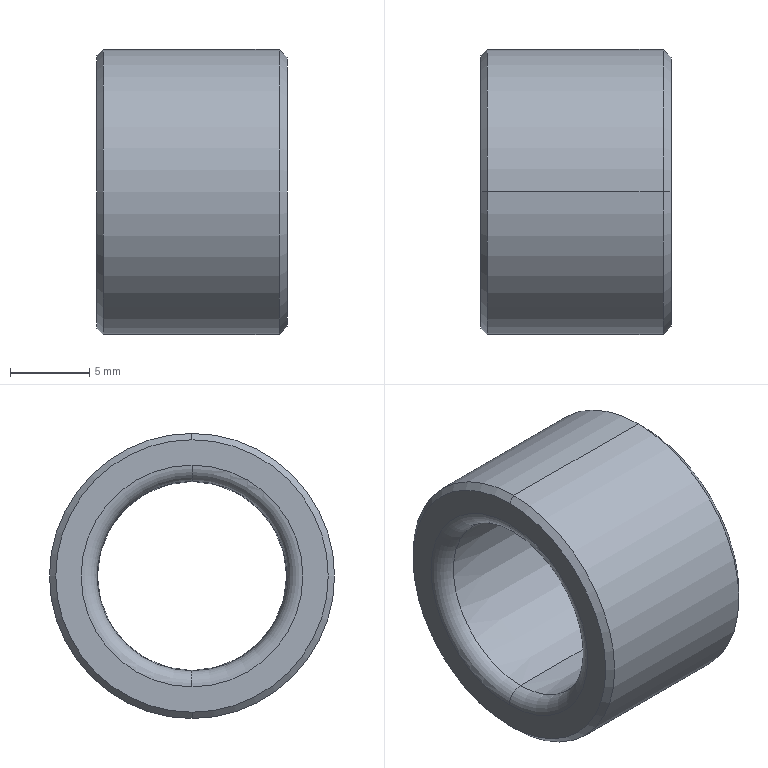Part | STEP file | SHBZ12_12_SHBZ12-100 | 1 solid | 16 faces | box 12 x 18 x 18 mm | volume 1675 mm3 | torus 6 | cone 6 | cylinder 2 | plane 2 | commonest cylinder face diameters 18 x2
STEP:
#1=CARTESIAN_POINT('',(11.,0.,-5.969));
#2=VERTEX_POINT('',#1);
#3=CARTESIAN_POINT('',(12.,0.,-6.969));
#4=VERTEX_POINT('',#3);
#5=CARTESIAN_POINT('',(11.,0.,-6.969));
#6=DIRECTION('',(0.,1.,0.));
#7=DIRECTION('',(0.,0.,1.));
#8=AXIS2_PLACEMENT_3D('',#5,#6,#7);
#9=CIRCLE('',#8,1.);
#10=EDGE_CURVE('',#2,#4,#9,.T.);
#11=ORIENTED_EDGE('',*,*,#10,.F.);
#12=CARTESIAN_POINT('',(11.,0.,5.969));
#13=VERTEX_POINT('',#12);
#14=CARTESIAN_POINT('',(11.,0.,0.));
#15=DIRECTION('',(-1.,0.,0.));
#16=DIRECTION('',(0.,0.,1.));
#17=AXIS2_PLACEMENT_3D('',#14,#15,#16);
#18=CIRCLE('',#17,5.969);
#19=EDGE_CURVE('',#2,#13,#18,.T.);
#20=ORIENTED_EDGE('',*,*,#19,.T.);
#21=CARTESIAN_POINT('',(12.,0.,6.969));
#22=VERTEX_POINT('',#21);
#23=CARTESIAN_POINT('',(11.,0.,6.969));
#24=DIRECTION('',(0.,-1.,0.));
#25=DIRECTION('',(0.,0.,-1.));
#26=AXIS2_PLACEMENT_3D('',#23,#24,#25);
#27=CIRCLE('',#26,1.);
#28=EDGE_CURVE('',#13,#22,#27,.T.);
#29=ORIENTED_EDGE('',*,*,#28,.T.);
#30=CARTESIAN_POINT('',(12.,0.,0.));
#31=DIRECTION('',(-1.,0.,0.));
#32=DIRECTION('',(0.,0.,1.));
#33=AXIS2_PLACEMENT_3D('',#30,#31,#32);
#34=CIRCLE('',#33,6.969);
#35=EDGE_CURVE('',#4,#22,#34,.T.);
#36=ORIENTED_EDGE('',*,*,#35,.F.);
#37=EDGE_LOOP('',(#11,#20,#29,#36));
#38=FACE_OUTER_BOUND('',#37,.T.);
#39=CARTESIAN_POINT('',(11.,0.,0.));
#40=DIRECTION('',(-1.,0.,0.));
#41=DIRECTION('',(0.,0.,1.));
#42=AXIS2_PLACEMENT_3D('',#39,#40,#41);
#43=TOROIDAL_SURFACE('',#42,6.969,1.);
#44=ADVANCED_FACE('',(#38),#43,.T.);
#45=ORIENTED_EDGE('',*,*,#28,.F.);
#46=CARTESIAN_POINT('',(11.,0.,0.));
#47=DIRECTION('',(-1.,0.,0.));
#48=DIRECTION('',(0.,0.,1.));
#49=AXIS2_PLACEMENT_3D('',#46,#47,#48);
#50=CIRCLE('',#49,5.969);
#51=EDGE_CURVE('',#13,#2,#50,.T.);
#52=ORIENTED_EDGE('',*,*,#51,.T.);
#53=ORIENTED_EDGE('',*,*,#10,.T.);
#54=CARTESIAN_POINT('',(12.,0.,0.));
#55=DIRECTION('',(-1.,0.,0.));
#56=DIRECTION('',(0.,0.,1.));
#57=AXIS2_PLACEMENT_3D('',#54,#55,#56);
#58=CIRCLE('',#57,6.969);
#59=EDGE_CURVE('',#22,#4,#58,.T.);
#60=ORIENTED_EDGE('',*,*,#59,.F.);
#61=EDGE_LOOP('',(#45,#52,#53,#60));
#62=FACE_OUTER_BOUND('',#61,.T.);
#63=CARTESIAN_POINT('',(11.,0.,0.));
#64=DIRECTION('',(-1.,0.,0.));
#65=DIRECTION('',(0.,0.,1.));
#66=AXIS2_PLACEMENT_3D('',#63,#64,#65);
#67=TOROIDAL_SURFACE('',#66,6.969,1.);
#68=ADVANCED_FACE('',(#62),#67,.T.);
#69=CARTESIAN_POINT('',(0.,0.,7.));
#70=VERTEX_POINT('',#69);
#71=CARTESIAN_POINT('',(0.,0.,-7.));
#72=VERTEX_POINT('',#71);
#73=CARTESIAN_POINT('',(0.,0.,0.));
#74=DIRECTION('',(-1.,0.,0.));
#75=DIRECTION('',(0.,0.,1.));
#76=AXIS2_PLACEMENT_3D('',#73,#74,#75);
#77=CIRCLE('',#76,7.);
#78=EDGE_CURVE('',#70,#72,#77,.T.);
#79=ORIENTED_EDGE('',*,*,#78,.T.);
#80=CARTESIAN_POINT('',(0.9969,0.,-6.));
#81=VERTEX_POINT('',#80);
#82=CARTESIAN_POINT('',(1.,0.,-7.));
#83=DIRECTION('',(0.,1.,0.));
#84=DIRECTION('',(0.,0.,1.));
#85=AXIS2_PLACEMENT_3D('',#82,#83,#84);
#86=CIRCLE('',#85,1.);
#87=EDGE_CURVE('',#72,#81,#86,.T.);
#88=ORIENTED_EDGE('',*,*,#87,.T.);
#89=CARTESIAN_POINT('',(0.9969,0.,6.));
#90=VERTEX_POINT('',#89);
#91=CARTESIAN_POINT('',(0.9969,0.,0.));
#92=DIRECTION('',(-1.,0.,0.));
#93=DIRECTION('',(0.,0.,1.));
#94=AXIS2_PLACEMENT_3D('',#91,#92,#93);
#95=CIRCLE('',#94,6.);
#96=EDGE_CURVE('',#90,#81,#95,.T.);
#97=ORIENTED_EDGE('',*,*,#96,.F.);
#98=CARTESIAN_POINT('',(1.,0.,7.));
#99=DIRECTION('',(0.,-1.,0.));
#100=DIRECTION('',(0.,0.,-1.));
#101=AXIS2_PLACEMENT_3D('',#98,#99,#100);
#102=CIRCLE('',#101,1.);
#103=EDGE_CURVE('',#70,#90,#102,.T.);
#104=ORIENTED_EDGE('',*,*,#103,.F.);
#105=EDGE_LOOP('',(#79,#88,#97,#104));
#106=FACE_OUTER_BOUND('',#105,.T.);
#107=CARTESIAN_POINT('',(1.,0.,0.));
#108=DIRECTION('',(-1.,0.,0.));
#109=DIRECTION('',(0.,0.,1.));
#110=AXIS2_PLACEMENT_3D('',#107,#108,#109);
#111=TOROIDAL_SURFACE('',#110,7.,1.);
#112=ADVANCED_FACE('',(#106),#111,.T.);
#113=CARTESIAN_POINT('',(10.997,0.,-5.969));
#114=VERTEX_POINT('',#113);
#115=CARTESIAN_POINT('',(10.997,0.,5.969));
#116=VERTEX_POINT('',#115);
#117=CARTESIAN_POINT('',(10.997,0.,0.));
#118=DIRECTION('',(-1.,0.,0.));
#119=DIRECTION('',(0.,0.,1.));
#120=AXIS2_PLACEMENT_3D('',#117,#118,#119);
#121=CIRCLE('',#120,5.969);
#122=EDGE_CURVE('',#114,#116,#121,.T.);
#123=ORIENTED_EDGE('',*,*,#122,.F.);
#124=CARTESIAN_POINT('',(0.9969,0.,-6.));
#125=DIRECTION('',(-1.,0.,-0.003115));
#126=VECTOR('',#125,1000.);
#127=LINE('',#124,#126);
#128=EDGE_CURVE('',#114,#81,#127,.T.);
#129=ORIENTED_EDGE('',*,*,#128,.T.);
#130=CARTESIAN_POINT('',(0.9969,0.,0.));
#131=DIRECTION('',(-1.,0.,0.));
#132=DIRECTION('',(0.,0.,1.));
#133=AXIS2_PLACEMENT_3D('',#130,#131,#132);
#134=CIRCLE('',#133,6.);
#135=EDGE_CURVE('',#81,#90,#134,.T.);
#136=ORIENTED_EDGE('',*,*,#135,.T.);
#137=CARTESIAN_POINT('',(0.9969,0.,6.));
#138=DIRECTION('',(-1.,0.,0.003115));
#139=VECTOR('',#138,1000.);
#140=LINE('',#137,#139);
#141=EDGE_CURVE('',#116,#90,#140,.T.);
#142=ORIENTED_EDGE('',*,*,#141,.F.);
#143=EDGE_LOOP('',(#123,#129,#136,#142));
#144=FACE_OUTER_BOUND('',#143,.T.);
#145=CARTESIAN_POINT('',(0.9969,0.,0.));
#146=DIRECTION('',(-1.,0.,0.));
#147=DIRECTION('',(0.,0.,1.));
#148=AXIS2_PLACEMENT_3D('',#145,#146,#147);
#149=CONICAL_SURFACE('',#148,6.,0.003115);
#150=ADVANCED_FACE('',(#144),#149,.F.);
#151=ORIENTED_EDGE('',*,*,#51,.F.);
#152=CARTESIAN_POINT('',(11.,0.,6.969));
#153=DIRECTION('',(0.,-1.,0.));
#154=DIRECTION('',(0.,0.,-1.));
#155=AXIS2_PLACEMENT_3D('',#152,#153,#154);
#156=CIRCLE('',#155,1.);
#157=EDGE_CURVE('',#116,#13,#156,.T.);
#158=ORIENTED_EDGE('',*,*,#157,.F.);
#159=CARTESIAN_POINT('',(10.997,0.,0.));
#160=DIRECTION('',(-1.,0.,0.));
#161=DIRECTION('',(0.,0.,1.));
#162=AXIS2_PLACEMENT_3D('',#159,#160,#161);
#163=CIRCLE('',#162,5.969);
#164=EDGE_CURVE('',#116,#114,#163,.T.);
#165=ORIENTED_EDGE('',*,*,#164,.T.);
#166=CARTESIAN_POINT('',(11.,0.,-6.969));
#167=DIRECTION('',(0.,1.,0.));
#168=DIRECTION('',(0.,0.,1.));
#169=AXIS2_PLACEMENT_3D('',#166,#167,#168);
#170=CIRCLE('',#169,1.);
#171=EDGE_CURVE('',#114,#2,#170,.T.);
#172=ORIENTED_EDGE('',*,*,#171,.T.);
#173=EDGE_LOOP('',(#151,#158,#165,#172));
#174=FACE_OUTER_BOUND('',#173,.T.);
#175=CARTESIAN_POINT('',(11.,0.,0.));
#176=DIRECTION('',(-1.,0.,0.));
#177=DIRECTION('',(0.,0.,1.));
#178=AXIS2_PLACEMENT_3D('',#175,#176,#177);
#179=TOROIDAL_SURFACE('',#178,6.969,1.);
#180=ADVANCED_FACE('',(#174),#179,.T.);
#181=CARTESIAN_POINT('',(12.,0.,8.5));
#182=VERTEX_POINT('',#181);
#183=CARTESIAN_POINT('',(12.,0.,-8.5));
#184=VERTEX_POINT('',#183);
#185=CARTESIAN_POINT('',(12.,0.,0.));
#186=DIRECTION('',(-1.,0.,0.));
#187=DIRECTION('',(0.,0.,1.));
#188=AXIS2_PLACEMENT_3D('',#185,#186,#187);
#189=CIRCLE('',#188,8.5);
#190=EDGE_CURVE('',#182,#184,#189,.T.);
#191=ORIENTED_EDGE('',*,*,#190,.T.);
#192=CARTESIAN_POINT('',(11.5,0.,-9.));
#193=VERTEX_POINT('',#192);
#194=CARTESIAN_POINT('',(12.,0.,-8.5));
#195=DIRECTION('',(-0.7071,0.,-0.7071));
#196=VECTOR('',#195,1000.);
#197=LINE('',#194,#196);
#198=EDGE_CURVE('',#184,#193,#197,.T.);
#199=ORIENTED_EDGE('',*,*,#198,.T.);
#200=CARTESIAN_POINT('',(11.5,0.,9.));
#201=VERTEX_POINT('',#200);
#202=CARTESIAN_POINT('',(11.5,0.,0.));
#203=DIRECTION('',(-1.,0.,0.));
#204=DIRECTION('',(0.,0.,1.));
#205=AXIS2_PLACEMENT_3D('',#202,#203,#204);
#206=CIRCLE('',#205,9.);
#207=EDGE_CURVE('',#201,#193,#206,.T.);
#208=ORIENTED_EDGE('',*,*,#207,.F.);
#209=CARTESIAN_POINT('',(12.,0.,8.5));
#210=DIRECTION('',(-0.7071,0.,0.7071));
#211=VECTOR('',#210,1000.);
#212=LINE('',#209,#211);
#213=EDGE_CURVE('',#182,#201,#212,.T.);
#214=ORIENTED_EDGE('',*,*,#213,.F.);
#215=EDGE_LOOP('',(#191,#199,#208,#214));
#216=FACE_OUTER_BOUND('',#215,.T.);
#217=CARTESIAN_POINT('',(12.,0.,0.));
#218=DIRECTION('',(-1.,0.,0.));
#219=DIRECTION('',(0.,0.,1.));
#220=AXIS2_PLACEMENT_3D('',#217,#218,#219);
#221=CONICAL_SURFACE('',#220,8.5,0.7854);
#222=ADVANCED_FACE('',(#216),#221,.T.);
#223=ORIENTED_EDGE('',*,*,#207,.T.);
#224=CARTESIAN_POINT('',(0.4,0.,-9.));
#225=VERTEX_POINT('',#224);
#226=CARTESIAN_POINT('',(10.,0.,-9.));
#227=DIRECTION('',(-1.,0.,0.));
#228=VECTOR('',#227,1000.);
#229=LINE('',#226,#228);
#230=EDGE_CURVE('',#193,#225,#229,.T.);
#231=ORIENTED_EDGE('',*,*,#230,.T.);
#232=CARTESIAN_POINT('',(0.4,0.,9.));
#233=VERTEX_POINT('',#232);
#234=CARTESIAN_POINT('',(0.4,0.,0.));
#235=DIRECTION('',(-1.,0.,0.));
#236=DIRECTION('',(0.,0.,1.));
#237=AXIS2_PLACEMENT_3D('',#234,#235,#236);
#238=CIRCLE('',#237,9.);
#239=EDGE_CURVE('',#233,#225,#238,.T.);
#240=ORIENTED_EDGE('',*,*,#239,.F.);
#241=CARTESIAN_POINT('',(10.,0.,9.));
#242=DIRECTION('',(-1.,0.,0.));
#243=VECTOR('',#242,1000.);
#244=LINE('',#241,#243);
#245=EDGE_CURVE('',#201,#233,#244,.T.);
#246=ORIENTED_EDGE('',*,*,#245,.F.);
#247=EDGE_LOOP('',(#223,#231,#240,#246));
#248=FACE_OUTER_BOUND('',#247,.T.);
#249=CARTESIAN_POINT('',(10.,0.,0.));
#250=DIRECTION('',(-1.,0.,0.));
#251=DIRECTION('',(0.,0.,1.));
#252=AXIS2_PLACEMENT_3D('',#249,#250,#251);
#253=CYLINDRICAL_SURFACE('',#252,9.);
#254=ADVANCED_FACE('',(#248),#253,.T.);
#255=CARTESIAN_POINT('',(0.,0.,8.6));
#256=VERTEX_POINT('',#255);
#257=CARTESIAN_POINT('',(0.,0.,-8.6));
#258=VERTEX_POINT('',#257);
#259=CARTESIAN_POINT('',(0.,0.,0.));
#260=DIRECTION('',(-1.,0.,0.));
#261=DIRECTION('',(0.,0.,1.));
#262=AXIS2_PLACEMENT_3D('',#259,#260,#261);
#263=CIRCLE('',#262,8.6);
#264=EDGE_CURVE('',#256,#258,#263,.T.);
#265=ORIENTED_EDGE('',*,*,#264,.F.);
#266=CARTESIAN_POINT('',(0.4,0.,9.));
#267=DIRECTION('',(0.7071,0.,0.7071));
#268=VECTOR('',#267,1000.);
#269=LINE('',#266,#268);
#270=EDGE_CURVE('',#256,#233,#269,.T.);
#271=ORIENTED_EDGE('',*,*,#270,.T.);
#272=ORIENTED_EDGE('',*,*,#239,.T.);
#273=CARTESIAN_POINT('',(0.4,0.,-9.));
#274=DIRECTION('',(0.7071,0.,-0.7071));
#275=VECTOR('',#274,1000.);
#276=LINE('',#273,#275);
#277=EDGE_CURVE('',#258,#225,#276,.T.);
#278=ORIENTED_EDGE('',*,*,#277,.F.);
#279=EDGE_LOOP('',(#265,#271,#272,#278));
#280=FACE_OUTER_BOUND('',#279,.T.);
#281=CARTESIAN_POINT('',(0.4,0.,0.));
#282=DIRECTION('',(1.,0.,0.));
#283=DIRECTION('',(0.,0.,-1.));
#284=AXIS2_PLACEMENT_3D('',#281,#282,#283);
#285=CONICAL_SURFACE('',#284,9.,0.7854);
#286=ADVANCED_FACE('',(#280),#285,.T.);
#287=ORIENTED_EDGE('',*,*,#270,.F.);
#288=CARTESIAN_POINT('',(0.,0.,0.));
#289=DIRECTION('',(-1.,0.,0.));
#290=DIRECTION('',(0.,0.,1.));
#291=AXIS2_PLACEMENT_3D('',#288,#289,#290);
#292=CIRCLE('',#291,8.6);
#293=EDGE_CURVE('',#258,#256,#292,.T.);
#294=ORIENTED_EDGE('',*,*,#293,.F.);
#295=ORIENTED_EDGE('',*,*,#277,.T.);
#296=CARTESIAN_POINT('',(0.4,0.,0.));
#297=DIRECTION('',(-1.,0.,0.));
#298=DIRECTION('',(0.,0.,1.));
#299=AXIS2_PLACEMENT_3D('',#296,#297,#298);
#300=CIRCLE('',#299,9.);
#301=EDGE_CURVE('',#225,#233,#300,.T.);
#302=ORIENTED_EDGE('',*,*,#301,.T.);
#303=EDGE_LOOP('',(#287,#294,#295,#302));
#304=FACE_OUTER_BOUND('',#303,.T.);
#305=CARTESIAN_POINT('',(0.4,0.,0.));
#306=DIRECTION('',(1.,0.,0.));
#307=DIRECTION('',(0.,0.,-1.));
#308=AXIS2_PLACEMENT_3D('',#305,#306,#307);
#309=CONICAL_SURFACE('',#308,9.,0.7854);
#310=ADVANCED_FACE('',(#304),#309,.T.);
#311=ORIENTED_EDGE('',*,*,#230,.F.);
#312=CARTESIAN_POINT('',(11.5,0.,0.));
#313=DIRECTION('',(-1.,0.,0.));
#314=DIRECTION('',(0.,0.,1.));
#315=AXIS2_PLACEMENT_3D('',#312,#313,#314);
#316=CIRCLE('',#315,9.);
#317=EDGE_CURVE('',#193,#201,#316,.T.);
#318=ORIENTED_EDGE('',*,*,#317,.T.);
#319=ORIENTED_EDGE('',*,*,#245,.T.);
#320=ORIENTED_EDGE('',*,*,#301,.F.);
#321=EDGE_LOOP('',(#311,#318,#319,#320));
#322=FACE_OUTER_BOUND('',#321,.T.);
#323=CARTESIAN_POINT('',(10.,0.,0.));
#324=DIRECTION('',(-1.,0.,0.));
#325=DIRECTION('',(0.,0.,1.));
#326=AXIS2_PLACEMENT_3D('',#323,#324,#325);
#327=CYLINDRICAL_SURFACE('',#326,9.);
#328=ADVANCED_FACE('',(#322),#327,.T.);
#329=ORIENTED_EDGE('',*,*,#198,.F.);
#330=CARTESIAN_POINT('',(12.,0.,0.));
#331=DIRECTION('',(-1.,0.,0.));
#332=DIRECTION('',(0.,0.,1.));
#333=AXIS2_PLACEMENT_3D('',#330,#331,#332);
#334=CIRCLE('',#333,8.5);
#335=EDGE_CURVE('',#184,#182,#334,.T.);
#336=ORIENTED_EDGE('',*,*,#335,.T.);
#337=ORIENTED_EDGE('',*,*,#213,.T.);
#338=ORIENTED_EDGE('',*,*,#317,.F.);
#339=EDGE_LOOP('',(#329,#336,#337,#338));
#340=FACE_OUTER_BOUND('',#339,.T.);
#341=CARTESIAN_POINT('',(12.,0.,0.));
#342=DIRECTION('',(-1.,0.,0.));
#343=DIRECTION('',(0.,0.,1.));
#344=AXIS2_PLACEMENT_3D('',#341,#342,#343);
#345=CONICAL_SURFACE('',#344,8.5,0.7854);
#346=ADVANCED_FACE('',(#340),#345,.T.);
#347=ORIENTED_EDGE('',*,*,#190,.F.);
#348=ORIENTED_EDGE('',*,*,#335,.F.);
#349=EDGE_LOOP('',(#347,#348));
#350=FACE_OUTER_BOUND('',#349,.T.);
#351=ORIENTED_EDGE('',*,*,#59,.T.);
#352=ORIENTED_EDGE('',*,*,#35,.T.);
#353=EDGE_LOOP('',(#351,#352));
#354=FACE_BOUND('',#353,.T.);
#355=CARTESIAN_POINT('',(12.,6.969,0.));
#356=DIRECTION('',(-1.,0.,0.));
#357=DIRECTION('',(0.,0.,1.));
#358=AXIS2_PLACEMENT_3D('',#355,#356,#357);
#359=PLANE('',#358);
#360=ADVANCED_FACE('',(#350,#354),#359,.F.);
#361=ORIENTED_EDGE('',*,*,#19,.F.);
#362=ORIENTED_EDGE('',*,*,#171,.F.);
#363=ORIENTED_EDGE('',*,*,#122,.T.);
#364=ORIENTED_EDGE('',*,*,#157,.T.);
#365=EDGE_LOOP('',(#361,#362,#363,#364));
#366=FACE_OUTER_BOUND('',#365,.T.);
#367=CARTESIAN_POINT('',(11.,0.,0.));
#368=DIRECTION('',(-1.,0.,0.));
#369=DIRECTION('',(0.,0.,1.));
#370=AXIS2_PLACEMENT_3D('',#367,#368,#369);
#371=TOROIDAL_SURFACE('',#370,6.969,1.);
#372=ADVANCED_FACE('',(#366),#371,.T.);
#373=ORIENTED_EDGE('',*,*,#128,.F.);
#374=ORIENTED_EDGE('',*,*,#164,.F.);
#375=ORIENTED_EDGE('',*,*,#141,.T.);
#376=ORIENTED_EDGE('',*,*,#96,.T.);
#377=EDGE_LOOP('',(#373,#374,#375,#376));
#378=FACE_OUTER_BOUND('',#377,.T.);
#379=CARTESIAN_POINT('',(0.9969,0.,0.));
#380=DIRECTION('',(-1.,0.,0.));
#381=DIRECTION('',(0.,0.,1.));
#382=AXIS2_PLACEMENT_3D('',#379,#380,#381);
#383=CONICAL_SURFACE('',#382,6.,0.003115);
#384=ADVANCED_FACE('',(#378),#383,.F.);
#385=ORIENTED_EDGE('',*,*,#87,.F.);
#386=CARTESIAN_POINT('',(0.,0.,0.));
#387=DIRECTION('',(-1.,0.,0.));
#388=DIRECTION('',(0.,0.,1.));
#389=AXIS2_PLACEMENT_3D('',#386,#387,#388);
#390=CIRCLE('',#389,7.);
#391=EDGE_CURVE('',#72,#70,#390,.T.);
#392=ORIENTED_EDGE('',*,*,#391,.T.);
#393=ORIENTED_EDGE('',*,*,#103,.T.);
#394=ORIENTED_EDGE('',*,*,#135,.F.);
#395=EDGE_LOOP('',(#385,#392,#393,#394));
#396=FACE_OUTER_BOUND('',#395,.T.);
#397=CARTESIAN_POINT('',(1.,0.,0.));
#398=DIRECTION('',(-1.,0.,0.));
#399=DIRECTION('',(0.,0.,1.));
#400=AXIS2_PLACEMENT_3D('',#397,#398,#399);
#401=TOROIDAL_SURFACE('',#400,7.,1.);
#402=ADVANCED_FACE('',(#396),#401,.T.);
#403=ORIENTED_EDGE('',*,*,#78,.F.);
#404=ORIENTED_EDGE('',*,*,#391,.F.);
#405=EDGE_LOOP('',(#403,#404));
#406=FACE_BOUND('',#405,.T.);
#407=ORIENTED_EDGE('',*,*,#293,.T.);
#408=ORIENTED_EDGE('',*,*,#264,.T.);
#409=EDGE_LOOP('',(#407,#408));
#410=FACE_OUTER_BOUND('',#409,.T.);
#411=CARTESIAN_POINT('',(0.,8.6,0.));
#412=DIRECTION('',(1.,0.,0.));
#413=DIRECTION('',(0.,0.,-1.));
#414=AXIS2_PLACEMENT_3D('',#411,#412,#413);
#415=PLANE('',#414);
#416=ADVANCED_FACE('',(#406,#410),#415,.F.);
#417=CLOSED_SHELL('',(#44,#68,#112,#150,#180,#222,#254,#286,#310,#328,#346,#360,#372,#384,#402,#416));
#418=MANIFOLD_SOLID_BREP('',#417);
#419=CARTESIAN_POINT('',(0.,0.,0.));
#420=DIRECTION('',(0.,0.,1.));
#421=DIRECTION('',(1.,0.,0.));
#422=AXIS2_PLACEMENT_3D('',#419,#420,#421);
#423=(LENGTH_UNIT()NAMED_UNIT(*)SI_UNIT(.MILLI.,.METRE.));
#424=UNCERTAINTY_MEASURE_WITH_UNIT(LENGTH_MEASURE(0.00001),#423,'','');
#425=(NAMED_UNIT(*)PLANE_ANGLE_UNIT()SI_UNIT($,.RADIAN.));
#426=(NAMED_UNIT(*)SI_UNIT($,.STERADIAN.)SOLID_ANGLE_UNIT());
#427=(GEOMETRIC_REPRESENTATION_CONTEXT(3)GLOBAL_UNCERTAINTY_ASSIGNED_CONTEXT((#424))GLOBAL_UNIT_ASSIGNED_CONTEXT((#423,#425,#426))REPRESENTATION_CONTEXT('',''));
#428=ADVANCED_BREP_SHAPE_REPRESENTATION('',(#418,#422),#427);